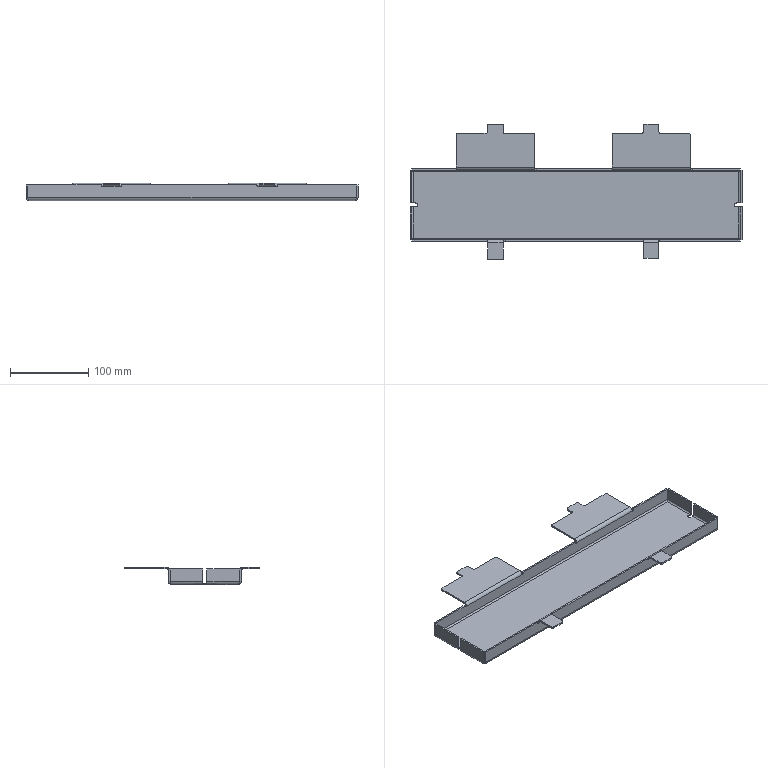Part | STEP file | 68341485 | 1 solid | 158 faces | box 425 x 174 x 22 mm | volume 133591 mm3 | plane 96 | cylinder 46 | spline 16 | commonest cylinder face diameters 4 x26 8 x10 3 x8 5 x2